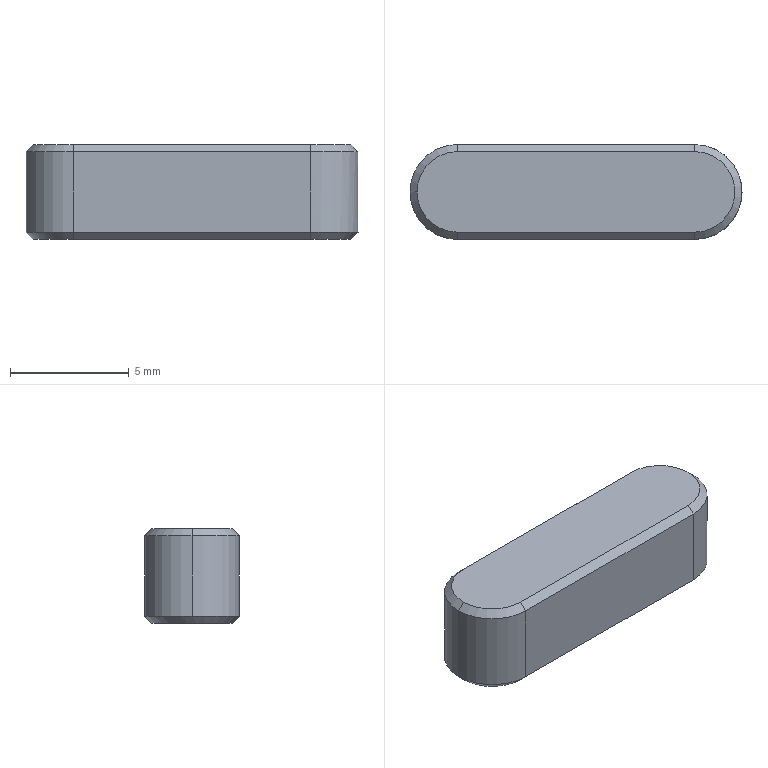Part | NX | features BREP 1 | 1 solid | 17 faces | box 14 x 4 x 4 mm | volume 207.391 mm3 | plane 8 | cone 6 | cylinder 3 | commonest cylinder face diameters 4 x3
STEP:
#1=CARTESIAN_POINT('',(-6.7,0.,2.));
#2=VERTEX_POINT('',#1);
#3=CARTESIAN_POINT('',(-5.,-1.7,2.));
#4=VERTEX_POINT('',#3);
#5=CARTESIAN_POINT('',(-5.,0.,2.));
#6=DIRECTION('',(0.,0.,1.));
#7=DIRECTION('',(1.,0.,0.));
#8=AXIS2_PLACEMENT_3D('',#5,#6,#7);
#9=CIRCLE('',#8,1.7);
#10=EDGE_CURVE('',#2,#4,#9,.T.);
#11=ORIENTED_EDGE('',*,*,#10,.F.);
#12=CARTESIAN_POINT('',(-7.,0.,1.7));
#13=VERTEX_POINT('',#12);
#14=CARTESIAN_POINT('',(-6.7,0.,2.));
#15=DIRECTION('',(-0.7071,0.,-0.7071));
#16=VECTOR('',#15,1000.);
#17=LINE('',#14,#16);
#18=EDGE_CURVE('',#2,#13,#17,.T.);
#19=ORIENTED_EDGE('',*,*,#18,.T.);
#20=CARTESIAN_POINT('',(-5.,-2.,1.7));
#21=VERTEX_POINT('',#20);
#22=CARTESIAN_POINT('',(-5.,0.,1.7));
#23=DIRECTION('',(0.,0.,-1.));
#24=DIRECTION('',(1.,0.,0.));
#25=AXIS2_PLACEMENT_3D('',#22,#23,#24);
#26=CIRCLE('',#25,2.);
#27=EDGE_CURVE('',#21,#13,#26,.T.);
#28=ORIENTED_EDGE('',*,*,#27,.F.);
#29=CARTESIAN_POINT('',(-5.,-2.,1.7));
#30=DIRECTION('',(0.,0.7071,0.7071));
#31=VECTOR('',#30,1000.);
#32=LINE('',#29,#31);
#33=EDGE_CURVE('',#21,#4,#32,.T.);
#34=ORIENTED_EDGE('',*,*,#33,.T.);
#35=EDGE_LOOP('',(#11,#19,#28,#34));
#36=FACE_BOUND('',#35,.T.);
#37=CARTESIAN_POINT('',(-5.,0.,2.));
#38=DIRECTION('',(0.,0.,-1.));
#39=DIRECTION('',(-1.,0.,0.));
#40=AXIS2_PLACEMENT_3D('',#37,#38,#39);
#41=CONICAL_SURFACE('',#40,1.7,0.7854);
#42=ADVANCED_FACE('',(#36),#41,.T.);
#43=CARTESIAN_POINT('',(6.7,0.,-2.));
#44=VERTEX_POINT('',#43);
#45=CARTESIAN_POINT('',(5.,-1.7,-2.));
#46=VERTEX_POINT('',#45);
#47=CARTESIAN_POINT('',(5.,0.,-2.));
#48=DIRECTION('',(0.,0.,-1.));
#49=DIRECTION('',(1.,0.,0.));
#50=AXIS2_PLACEMENT_3D('',#47,#48,#49);
#51=CIRCLE('',#50,1.7);
#52=EDGE_CURVE('',#44,#46,#51,.T.);
#53=ORIENTED_EDGE('',*,*,#52,.F.);
#54=CARTESIAN_POINT('',(7.,0.,-1.7));
#55=VERTEX_POINT('',#54);
#56=CARTESIAN_POINT('',(7.,0.,-1.7));
#57=DIRECTION('',(0.7071,0.,0.7071));
#58=VECTOR('',#57,1000.);
#59=LINE('',#56,#58);
#60=EDGE_CURVE('',#44,#55,#59,.T.);
#61=ORIENTED_EDGE('',*,*,#60,.T.);
#62=CARTESIAN_POINT('',(5.,-2.,-1.7));
#63=VERTEX_POINT('',#62);
#64=CARTESIAN_POINT('',(5.,0.,-1.7));
#65=DIRECTION('',(0.,0.,1.));
#66=DIRECTION('',(1.,0.,0.));
#67=AXIS2_PLACEMENT_3D('',#64,#65,#66);
#68=CIRCLE('',#67,2.);
#69=EDGE_CURVE('',#63,#55,#68,.T.);
#70=ORIENTED_EDGE('',*,*,#69,.F.);
#71=CARTESIAN_POINT('',(5.,-2.,-1.7));
#72=DIRECTION('',(0.,0.7071,-0.7071));
#73=VECTOR('',#72,1000.);
#74=LINE('',#71,#73);
#75=EDGE_CURVE('',#63,#46,#74,.T.);
#76=ORIENTED_EDGE('',*,*,#75,.T.);
#77=EDGE_LOOP('',(#53,#61,#70,#76));
#78=FACE_BOUND('',#77,.T.);
#79=CARTESIAN_POINT('',(5.,0.,-1.7));
#80=DIRECTION('',(0.,0.,1.));
#81=DIRECTION('',(1.,0.,0.));
#82=AXIS2_PLACEMENT_3D('',#79,#80,#81);
#83=CONICAL_SURFACE('',#82,2.,0.7854);
#84=ADVANCED_FACE('',(#78),#83,.T.);
#85=ORIENTED_EDGE('',*,*,#27,.T.);
#86=CARTESIAN_POINT('',(-7.,0.,-1.7));
#87=VERTEX_POINT('',#86);
#88=CARTESIAN_POINT('',(-7.,0.,2.));
#89=DIRECTION('',(0.,0.,-1.));
#90=VECTOR('',#89,1000.);
#91=LINE('',#88,#90);
#92=EDGE_CURVE('',#13,#87,#91,.T.);
#93=ORIENTED_EDGE('',*,*,#92,.T.);
#94=CARTESIAN_POINT('',(-5.,-2.,-1.7));
#95=VERTEX_POINT('',#94);
#96=CARTESIAN_POINT('',(-5.,0.,-1.7));
#97=DIRECTION('',(0.,0.,1.));
#98=DIRECTION('',(1.,0.,0.));
#99=AXIS2_PLACEMENT_3D('',#96,#97,#98);
#100=CIRCLE('',#99,2.);
#101=EDGE_CURVE('',#87,#95,#100,.T.);
#102=ORIENTED_EDGE('',*,*,#101,.T.);
#103=CARTESIAN_POINT('',(-5.,-2.,2.));
#104=DIRECTION('',(0.,0.,-1.));
#105=VECTOR('',#104,1000.);
#106=LINE('',#103,#105);
#107=EDGE_CURVE('',#21,#95,#106,.T.);
#108=ORIENTED_EDGE('',*,*,#107,.F.);
#109=EDGE_LOOP('',(#85,#93,#102,#108));
#110=FACE_BOUND('',#109,.T.);
#111=CARTESIAN_POINT('',(-5.,0.,2.));
#112=DIRECTION('',(0.,0.,-1.));
#113=DIRECTION('',(-1.,0.,0.));
#114=AXIS2_PLACEMENT_3D('',#111,#112,#113);
#115=CYLINDRICAL_SURFACE('',#114,2.);
#116=ADVANCED_FACE('',(#110),#115,.T.);
#117=ORIENTED_EDGE('',*,*,#92,.F.);
#118=CARTESIAN_POINT('',(-5.,2.,1.7));
#119=VERTEX_POINT('',#118);
#120=CARTESIAN_POINT('',(-5.,0.,1.7));
#121=DIRECTION('',(0.,0.,-1.));
#122=DIRECTION('',(1.,0.,0.));
#123=AXIS2_PLACEMENT_3D('',#120,#121,#122);
#124=CIRCLE('',#123,2.);
#125=EDGE_CURVE('',#13,#119,#124,.T.);
#126=ORIENTED_EDGE('',*,*,#125,.T.);
#127=CARTESIAN_POINT('',(-5.,2.,-1.7));
#128=VERTEX_POINT('',#127);
#129=CARTESIAN_POINT('',(-5.,2.,2.));
#130=DIRECTION('',(0.,0.,-1.));
#131=VECTOR('',#130,1000.);
#132=LINE('',#129,#131);
#133=EDGE_CURVE('',#119,#128,#132,.T.);
#134=ORIENTED_EDGE('',*,*,#133,.T.);
#135=CARTESIAN_POINT('',(-5.,0.,-1.7));
#136=DIRECTION('',(0.,0.,1.));
#137=DIRECTION('',(1.,0.,0.));
#138=AXIS2_PLACEMENT_3D('',#135,#136,#137);
#139=CIRCLE('',#138,2.);
#140=EDGE_CURVE('',#128,#87,#139,.T.);
#141=ORIENTED_EDGE('',*,*,#140,.T.);
#142=EDGE_LOOP('',(#117,#126,#134,#141));
#143=FACE_BOUND('',#142,.T.);
#144=CARTESIAN_POINT('',(-5.,0.,2.));
#145=DIRECTION('',(0.,0.,-1.));
#146=DIRECTION('',(-1.,0.,0.));
#147=AXIS2_PLACEMENT_3D('',#144,#145,#146);
#148=CYLINDRICAL_SURFACE('',#147,2.);
#149=ADVANCED_FACE('',(#143),#148,.T.);
#150=ORIENTED_EDGE('',*,*,#107,.T.);
#151=CARTESIAN_POINT('',(-5.,-2.,-1.7));
#152=DIRECTION('',(1.,0.,0.));
#153=VECTOR('',#152,1000.);
#154=LINE('',#151,#153);
#155=EDGE_CURVE('',#95,#63,#154,.T.);
#156=ORIENTED_EDGE('',*,*,#155,.T.);
#157=CARTESIAN_POINT('',(5.,-2.,1.7));
#158=VERTEX_POINT('',#157);
#159=CARTESIAN_POINT('',(5.,-2.,2.));
#160=DIRECTION('',(0.,0.,-1.));
#161=VECTOR('',#160,1000.);
#162=LINE('',#159,#161);
#163=EDGE_CURVE('',#158,#63,#162,.T.);
#164=ORIENTED_EDGE('',*,*,#163,.F.);
#165=CARTESIAN_POINT('',(-5.,-2.,1.7));
#166=DIRECTION('',(-1.,0.,0.));
#167=VECTOR('',#166,1000.);
#168=LINE('',#165,#167);
#169=EDGE_CURVE('',#158,#21,#168,.T.);
#170=ORIENTED_EDGE('',*,*,#169,.T.);
#171=EDGE_LOOP('',(#150,#156,#164,#170));
#172=FACE_BOUND('',#171,.T.);
#173=CARTESIAN_POINT('',(-5.,-2.,2.));
#174=DIRECTION('',(0.,1.,0.));
#175=DIRECTION('',(1.,0.,0.));
#176=AXIS2_PLACEMENT_3D('',#173,#174,#175);
#177=PLANE('',#176);
#178=ADVANCED_FACE('',(#172),#177,.F.);
#179=ORIENTED_EDGE('',*,*,#163,.T.);
#180=ORIENTED_EDGE('',*,*,#69,.T.);
#181=CARTESIAN_POINT('',(5.,2.,-1.7));
#182=VERTEX_POINT('',#181);
#183=CARTESIAN_POINT('',(5.,0.,-1.7));
#184=DIRECTION('',(0.,0.,1.));
#185=DIRECTION('',(1.,0.,0.));
#186=AXIS2_PLACEMENT_3D('',#183,#184,#185);
#187=CIRCLE('',#186,2.);
#188=EDGE_CURVE('',#55,#182,#187,.T.);
#189=ORIENTED_EDGE('',*,*,#188,.T.);
#190=CARTESIAN_POINT('',(5.,2.,1.7));
#191=VERTEX_POINT('',#190);
#192=CARTESIAN_POINT('',(5.,2.,2.));
#193=DIRECTION('',(0.,0.,-1.));
#194=VECTOR('',#193,1000.);
#195=LINE('',#192,#194);
#196=EDGE_CURVE('',#191,#182,#195,.T.);
#197=ORIENTED_EDGE('',*,*,#196,.F.);
#198=CARTESIAN_POINT('',(5.,0.,1.7));
#199=DIRECTION('',(0.,0.,-1.));
#200=DIRECTION('',(1.,0.,0.));
#201=AXIS2_PLACEMENT_3D('',#198,#199,#200);
#202=CIRCLE('',#201,2.);
#203=EDGE_CURVE('',#191,#158,#202,.T.);
#204=ORIENTED_EDGE('',*,*,#203,.T.);
#205=EDGE_LOOP('',(#179,#180,#189,#197,#204));
#206=FACE_BOUND('',#205,.T.);
#207=CARTESIAN_POINT('',(5.,0.,2.));
#208=DIRECTION('',(0.,0.,-1.));
#209=DIRECTION('',(-1.,0.,0.));
#210=AXIS2_PLACEMENT_3D('',#207,#208,#209);
#211=CYLINDRICAL_SURFACE('',#210,2.);
#212=ADVANCED_FACE('',(#206),#211,.T.);
#213=ORIENTED_EDGE('',*,*,#196,.T.);
#214=CARTESIAN_POINT('',(-5.,2.,-1.7));
#215=DIRECTION('',(-1.,0.,0.));
#216=VECTOR('',#215,1000.);
#217=LINE('',#214,#216);
#218=EDGE_CURVE('',#182,#128,#217,.T.);
#219=ORIENTED_EDGE('',*,*,#218,.T.);
#220=ORIENTED_EDGE('',*,*,#133,.F.);
#221=CARTESIAN_POINT('',(5.,2.,1.7));
#222=DIRECTION('',(1.,0.,0.));
#223=VECTOR('',#222,1000.);
#224=LINE('',#221,#223);
#225=EDGE_CURVE('',#119,#191,#224,.T.);
#226=ORIENTED_EDGE('',*,*,#225,.T.);
#227=EDGE_LOOP('',(#213,#219,#220,#226));
#228=FACE_BOUND('',#227,.T.);
#229=CARTESIAN_POINT('',(-5.,2.,2.));
#230=DIRECTION('',(0.,-1.,0.));
#231=DIRECTION('',(0.,0.,-1.));
#232=AXIS2_PLACEMENT_3D('',#229,#230,#231);
#233=PLANE('',#232);
#234=ADVANCED_FACE('',(#228),#233,.F.);
#235=CARTESIAN_POINT('',(5.,-1.7,2.));
#236=VERTEX_POINT('',#235);
#237=CARTESIAN_POINT('',(5.,1.7,2.));
#238=VERTEX_POINT('',#237);
#239=CARTESIAN_POINT('',(5.,0.,2.));
#240=DIRECTION('',(0.,0.,1.));
#241=DIRECTION('',(1.,0.,0.));
#242=AXIS2_PLACEMENT_3D('',#239,#240,#241);
#243=CIRCLE('',#242,1.7);
#244=EDGE_CURVE('',#236,#238,#243,.T.);
#245=ORIENTED_EDGE('',*,*,#244,.T.);
#246=CARTESIAN_POINT('',(-5.,1.7,2.));
#247=VERTEX_POINT('',#246);
#248=CARTESIAN_POINT('',(-5.,1.7,2.));
#249=DIRECTION('',(-1.,0.,0.));
#250=VECTOR('',#249,1000.);
#251=LINE('',#248,#250);
#252=EDGE_CURVE('',#238,#247,#251,.T.);
#253=ORIENTED_EDGE('',*,*,#252,.T.);
#254=CARTESIAN_POINT('',(-5.,0.,2.));
#255=DIRECTION('',(0.,0.,1.));
#256=DIRECTION('',(1.,0.,0.));
#257=AXIS2_PLACEMENT_3D('',#254,#255,#256);
#258=CIRCLE('',#257,1.7);
#259=EDGE_CURVE('',#247,#2,#258,.T.);
#260=ORIENTED_EDGE('',*,*,#259,.T.);
#261=ORIENTED_EDGE('',*,*,#10,.T.);
#262=CARTESIAN_POINT('',(5.,-1.7,2.));
#263=DIRECTION('',(1.,0.,0.));
#264=VECTOR('',#263,1000.);
#265=LINE('',#262,#264);
#266=EDGE_CURVE('',#4,#236,#265,.T.);
#267=ORIENTED_EDGE('',*,*,#266,.T.);
#268=EDGE_LOOP('',(#245,#253,#260,#261,#267));
#269=FACE_BOUND('',#268,.T.);
#270=CARTESIAN_POINT('',(-5.,0.,2.));
#271=DIRECTION('',(0.,0.,1.));
#272=DIRECTION('',(1.,0.,0.));
#273=AXIS2_PLACEMENT_3D('',#270,#271,#272);
#274=PLANE('',#273);
#275=ADVANCED_FACE('',(#269),#274,.T.);
#276=CARTESIAN_POINT('',(-5.,-1.7,-2.));
#277=VERTEX_POINT('',#276);
#278=CARTESIAN_POINT('',(-5.,1.7,-2.));
#279=VERTEX_POINT('',#278);
#280=CARTESIAN_POINT('',(-5.,0.,-2.));
#281=DIRECTION('',(0.,0.,-1.));
#282=DIRECTION('',(1.,0.,0.));
#283=AXIS2_PLACEMENT_3D('',#280,#281,#282);
#284=CIRCLE('',#283,1.7);
#285=EDGE_CURVE('',#277,#279,#284,.T.);
#286=ORIENTED_EDGE('',*,*,#285,.T.);
#287=CARTESIAN_POINT('',(5.,1.7,-2.));
#288=VERTEX_POINT('',#287);
#289=CARTESIAN_POINT('',(-5.,1.7,-2.));
#290=DIRECTION('',(1.,0.,0.));
#291=VECTOR('',#290,1000.);
#292=LINE('',#289,#291);
#293=EDGE_CURVE('',#279,#288,#292,.T.);
#294=ORIENTED_EDGE('',*,*,#293,.T.);
#295=CARTESIAN_POINT('',(5.,0.,-2.));
#296=DIRECTION('',(0.,0.,-1.));
#297=DIRECTION('',(1.,0.,0.));
#298=AXIS2_PLACEMENT_3D('',#295,#296,#297);
#299=CIRCLE('',#298,1.7);
#300=EDGE_CURVE('',#288,#44,#299,.T.);
#301=ORIENTED_EDGE('',*,*,#300,.T.);
#302=ORIENTED_EDGE('',*,*,#52,.T.);
#303=CARTESIAN_POINT('',(-5.,-1.7,-2.));
#304=DIRECTION('',(-1.,0.,0.));
#305=VECTOR('',#304,1000.);
#306=LINE('',#303,#305);
#307=EDGE_CURVE('',#46,#277,#306,.T.);
#308=ORIENTED_EDGE('',*,*,#307,.T.);
#309=EDGE_LOOP('',(#286,#294,#301,#302,#308));
#310=FACE_BOUND('',#309,.T.);
#311=CARTESIAN_POINT('',(-5.,0.,-2.));
#312=DIRECTION('',(0.,0.,1.));
#313=DIRECTION('',(1.,0.,0.));
#314=AXIS2_PLACEMENT_3D('',#311,#312,#313);
#315=PLANE('',#314);
#316=ADVANCED_FACE('',(#310),#315,.F.);
#317=CARTESIAN_POINT('',(-5.,-1.7,-2.));
#318=DIRECTION('',(0.,-0.7071,0.7071));
#319=VECTOR('',#318,1000.);
#320=LINE('',#317,#319);
#321=EDGE_CURVE('',#277,#95,#320,.T.);
#322=ORIENTED_EDGE('',*,*,#321,.F.);
#323=ORIENTED_EDGE('',*,*,#307,.F.);
#324=ORIENTED_EDGE('',*,*,#75,.F.);
#325=ORIENTED_EDGE('',*,*,#155,.F.);
#326=EDGE_LOOP('',(#322,#323,#324,#325));
#327=FACE_BOUND('',#326,.T.);
#328=CARTESIAN_POINT('',(-5.,-2.,-1.7));
#329=DIRECTION('',(0.,0.7071,0.7071));
#330=DIRECTION('',(1.,0.,0.));
#331=AXIS2_PLACEMENT_3D('',#328,#329,#330);
#332=PLANE('',#331);
#333=ADVANCED_FACE('',(#327),#332,.F.);
#334=ORIENTED_EDGE('',*,*,#60,.F.);
#335=ORIENTED_EDGE('',*,*,#300,.F.);
#336=CARTESIAN_POINT('',(5.,2.,-1.7));
#337=DIRECTION('',(0.,-0.7071,-0.7071));
#338=VECTOR('',#337,1000.);
#339=LINE('',#336,#338);
#340=EDGE_CURVE('',#182,#288,#339,.T.);
#341=ORIENTED_EDGE('',*,*,#340,.F.);
#342=ORIENTED_EDGE('',*,*,#188,.F.);
#343=EDGE_LOOP('',(#334,#335,#341,#342));
#344=FACE_BOUND('',#343,.T.);
#345=CARTESIAN_POINT('',(5.,0.,-1.7));
#346=DIRECTION('',(0.,0.,1.));
#347=DIRECTION('',(1.,0.,0.));
#348=AXIS2_PLACEMENT_3D('',#345,#346,#347);
#349=CONICAL_SURFACE('',#348,2.,0.7854);
#350=ADVANCED_FACE('',(#344),#349,.T.);
#351=ORIENTED_EDGE('',*,*,#321,.T.);
#352=ORIENTED_EDGE('',*,*,#101,.F.);
#353=ORIENTED_EDGE('',*,*,#140,.F.);
#354=CARTESIAN_POINT('',(-5.,1.7,-2.));
#355=DIRECTION('',(0.,0.7071,0.7071));
#356=VECTOR('',#355,1000.);
#357=LINE('',#354,#356);
#358=EDGE_CURVE('',#279,#128,#357,.T.);
#359=ORIENTED_EDGE('',*,*,#358,.F.);
#360=ORIENTED_EDGE('',*,*,#285,.F.);
#361=EDGE_LOOP('',(#351,#352,#353,#359,#360));
#362=FACE_BOUND('',#361,.T.);
#363=CARTESIAN_POINT('',(-5.,0.,-1.7));
#364=DIRECTION('',(0.,0.,1.));
#365=DIRECTION('',(1.,0.,0.));
#366=AXIS2_PLACEMENT_3D('',#363,#364,#365);
#367=CONICAL_SURFACE('',#366,2.,0.7854);
#368=ADVANCED_FACE('',(#362),#367,.T.);
#369=ORIENTED_EDGE('',*,*,#340,.T.);
#370=ORIENTED_EDGE('',*,*,#293,.F.);
#371=ORIENTED_EDGE('',*,*,#358,.T.);
#372=ORIENTED_EDGE('',*,*,#218,.F.);
#373=EDGE_LOOP('',(#369,#370,#371,#372));
#374=FACE_BOUND('',#373,.T.);
#375=CARTESIAN_POINT('',(-5.,2.,-1.7));
#376=DIRECTION('',(0.,-0.7071,0.7071));
#377=DIRECTION('',(-1.,0.,0.));
#378=AXIS2_PLACEMENT_3D('',#375,#376,#377);
#379=PLANE('',#378);
#380=ADVANCED_FACE('',(#374),#379,.F.);
#381=ORIENTED_EDGE('',*,*,#33,.F.);
#382=ORIENTED_EDGE('',*,*,#169,.F.);
#383=CARTESIAN_POINT('',(5.,-1.7,2.));
#384=DIRECTION('',(0.,-0.7071,-0.7071));
#385=VECTOR('',#384,1000.);
#386=LINE('',#383,#385);
#387=EDGE_CURVE('',#236,#158,#386,.T.);
#388=ORIENTED_EDGE('',*,*,#387,.F.);
#389=ORIENTED_EDGE('',*,*,#266,.F.);
#390=EDGE_LOOP('',(#381,#382,#388,#389));
#391=FACE_BOUND('',#390,.T.);
#392=CARTESIAN_POINT('',(-5.,-1.7,2.));
#393=DIRECTION('',(0.,-0.7071,0.7071));
#394=DIRECTION('',(-1.,0.,0.));
#395=AXIS2_PLACEMENT_3D('',#392,#393,#394);
#396=PLANE('',#395);
#397=ADVANCED_FACE('',(#391),#396,.T.);
#398=ORIENTED_EDGE('',*,*,#387,.T.);
#399=ORIENTED_EDGE('',*,*,#203,.F.);
#400=CARTESIAN_POINT('',(5.,1.7,2.));
#401=DIRECTION('',(0.,0.7071,-0.7071));
#402=VECTOR('',#401,1000.);
#403=LINE('',#400,#402);
#404=EDGE_CURVE('',#238,#191,#403,.T.);
#405=ORIENTED_EDGE('',*,*,#404,.F.);
#406=ORIENTED_EDGE('',*,*,#244,.F.);
#407=EDGE_LOOP('',(#398,#399,#405,#406));
#408=FACE_BOUND('',#407,.T.);
#409=CARTESIAN_POINT('',(5.,0.,2.));
#410=DIRECTION('',(0.,0.,-1.));
#411=DIRECTION('',(-1.,0.,0.));
#412=AXIS2_PLACEMENT_3D('',#409,#410,#411);
#413=CONICAL_SURFACE('',#412,1.7,0.7854);
#414=ADVANCED_FACE('',(#408),#413,.T.);
#415=ORIENTED_EDGE('',*,*,#18,.F.);
#416=ORIENTED_EDGE('',*,*,#259,.F.);
#417=CARTESIAN_POINT('',(-5.,2.,1.7));
#418=DIRECTION('',(0.,-0.7071,0.7071));
#419=VECTOR('',#418,1000.);
#420=LINE('',#417,#419);
#421=EDGE_CURVE('',#119,#247,#420,.T.);
#422=ORIENTED_EDGE('',*,*,#421,.F.);
#423=ORIENTED_EDGE('',*,*,#125,.F.);
#424=EDGE_LOOP('',(#415,#416,#422,#423));
#425=FACE_BOUND('',#424,.T.);
#426=CARTESIAN_POINT('',(-5.,0.,2.));
#427=DIRECTION('',(0.,0.,-1.));
#428=DIRECTION('',(-1.,0.,0.));
#429=AXIS2_PLACEMENT_3D('',#426,#427,#428);
#430=CONICAL_SURFACE('',#429,1.7,0.7854);
#431=ADVANCED_FACE('',(#425),#430,.T.);
#432=ORIENTED_EDGE('',*,*,#404,.T.);
#433=ORIENTED_EDGE('',*,*,#225,.F.);
#434=ORIENTED_EDGE('',*,*,#421,.T.);
#435=ORIENTED_EDGE('',*,*,#252,.F.);
#436=EDGE_LOOP('',(#432,#433,#434,#435));
#437=FACE_BOUND('',#436,.T.);
#438=CARTESIAN_POINT('',(-5.,1.7,2.));
#439=DIRECTION('',(0.,0.7071,0.7071));
#440=DIRECTION('',(1.,0.,0.));
#441=AXIS2_PLACEMENT_3D('',#438,#439,#440);
#442=PLANE('',#441);
#443=ADVANCED_FACE('',(#437),#442,.T.);
#444=CLOSED_SHELL('',(#42,#84,#116,#149,#178,#212,#234,#275,#316,#333,#350,#368,#380,#397,#414,#431,#443));
#445=MANIFOLD_SOLID_BREP('',#444);
#446=(LENGTH_UNIT()NAMED_UNIT(*)SI_UNIT(.MILLI.,.METRE.));
#447=UNCERTAINTY_MEASURE_WITH_UNIT(LENGTH_MEASURE(0.00001),#446,'','');
#448=(NAMED_UNIT(*)PLANE_ANGLE_UNIT()SI_UNIT($,.RADIAN.));
#449=(NAMED_UNIT(*)SI_UNIT($,.STERADIAN.)SOLID_ANGLE_UNIT());
#450=(GEOMETRIC_REPRESENTATION_CONTEXT(3)GLOBAL_UNCERTAINTY_ASSIGNED_CONTEXT((#447))GLOBAL_UNIT_ASSIGNED_CONTEXT((#446,#448,#449))REPRESENTATION_CONTEXT('',''));
#451=ADVANCED_BREP_SHAPE_REPRESENTATION('',(#445),#450);